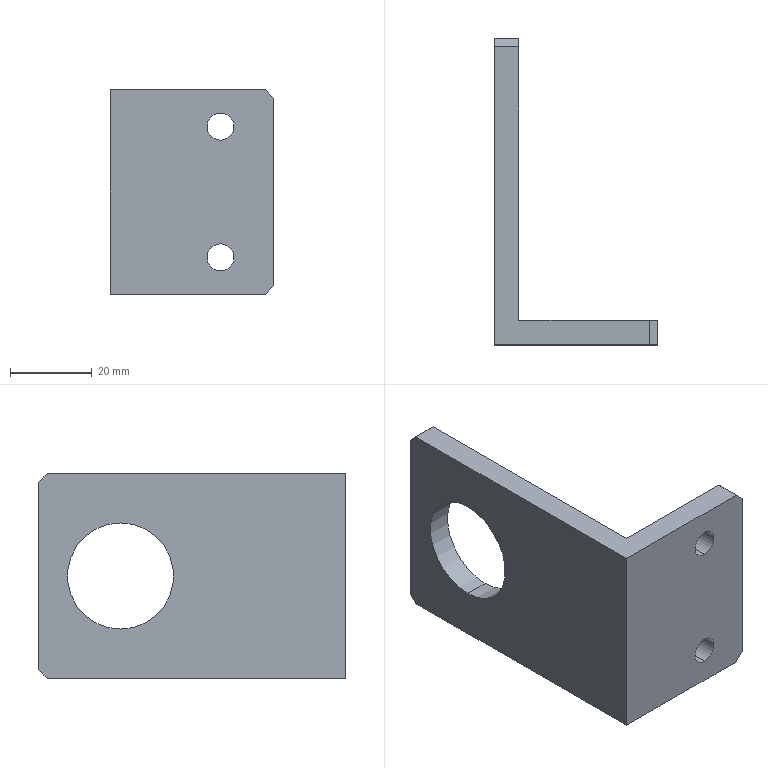Part | SolidWorks | features HoleWzd 2, Chamfer 1, Extrusion 1 | 1 solid | 18 faces | box 40 x 75 x 50 mm | volume 29056 mm3 | plane 12 | cylinder 6 | commonest cylinder face diameters 6.6 x4 26 x2
STEP:
#1=CARTESIAN_POINT('',(-13.82,-27.594,5.7));
#2=VERTEX_POINT('',#1);
#3=CARTESIAN_POINT('',(-13.82,-27.594,12.3));
#4=VERTEX_POINT('',#3);
#5=CARTESIAN_POINT('',(-13.82,-27.594,9.));
#6=DIRECTION('',(0.,1.,0.));
#7=DIRECTION('',(0.,0.,1.));
#8=AXIS2_PLACEMENT_3D('',#5,#6,#7);
#9=CIRCLE('',#8,3.3);
#10=EDGE_CURVE('',#2,#4,#9,.T.);
#11=ORIENTED_EDGE('',*,*,#10,.F.);
#12=CARTESIAN_POINT('',(-13.82,-21.594,5.7));
#13=VERTEX_POINT('',#12);
#14=CARTESIAN_POINT('',(-13.82,-21.594,5.7));
#15=DIRECTION('',(0.,1.,0.));
#16=VECTOR('',#15,1000.);
#17=LINE('',#14,#16);
#18=EDGE_CURVE('',#2,#13,#17,.T.);
#19=ORIENTED_EDGE('',*,*,#18,.T.);
#20=CARTESIAN_POINT('',(-13.82,-21.594,12.3));
#21=VERTEX_POINT('',#20);
#22=CARTESIAN_POINT('',(-13.82,-21.594,9.));
#23=DIRECTION('',(0.,1.,0.));
#24=DIRECTION('',(0.,0.,1.));
#25=AXIS2_PLACEMENT_3D('',#22,#23,#24);
#26=CIRCLE('',#25,3.3);
#27=EDGE_CURVE('',#13,#21,#26,.T.);
#28=ORIENTED_EDGE('',*,*,#27,.T.);
#29=CARTESIAN_POINT('',(-13.82,-21.594,12.3));
#30=DIRECTION('',(0.,1.,0.));
#31=VECTOR('',#30,1000.);
#32=LINE('',#29,#31);
#33=EDGE_CURVE('',#4,#21,#32,.T.);
#34=ORIENTED_EDGE('',*,*,#33,.F.);
#35=EDGE_LOOP('',(#11,#19,#28,#34));
#36=FACE_OUTER_BOUND('',#35,.T.);
#37=CARTESIAN_POINT('',(-13.82,-21.594,9.));
#38=DIRECTION('',(0.,1.,0.));
#39=DIRECTION('',(0.,0.,1.));
#40=AXIS2_PLACEMENT_3D('',#37,#38,#39);
#41=CYLINDRICAL_SURFACE('',#40,3.3);
#42=ADVANCED_FACE('',(#36),#41,.F.);
#43=CARTESIAN_POINT('',(-13.82,-27.594,37.7));
#44=VERTEX_POINT('',#43);
#45=CARTESIAN_POINT('',(-13.82,-27.594,44.3));
#46=VERTEX_POINT('',#45);
#47=CARTESIAN_POINT('',(-13.82,-27.594,41.));
#48=DIRECTION('',(0.,1.,0.));
#49=DIRECTION('',(0.,0.,1.));
#50=AXIS2_PLACEMENT_3D('',#47,#48,#49);
#51=CIRCLE('',#50,3.3);
#52=EDGE_CURVE('',#44,#46,#51,.T.);
#53=ORIENTED_EDGE('',*,*,#52,.F.);
#54=CARTESIAN_POINT('',(-13.82,-21.594,37.7));
#55=VERTEX_POINT('',#54);
#56=CARTESIAN_POINT('',(-13.82,-21.594,37.7));
#57=DIRECTION('',(0.,1.,0.));
#58=VECTOR('',#57,1000.);
#59=LINE('',#56,#58);
#60=EDGE_CURVE('',#44,#55,#59,.T.);
#61=ORIENTED_EDGE('',*,*,#60,.T.);
#62=CARTESIAN_POINT('',(-13.82,-21.594,44.3));
#63=VERTEX_POINT('',#62);
#64=CARTESIAN_POINT('',(-13.82,-21.594,41.));
#65=DIRECTION('',(0.,1.,0.));
#66=DIRECTION('',(0.,0.,1.));
#67=AXIS2_PLACEMENT_3D('',#64,#65,#66);
#68=CIRCLE('',#67,3.3);
#69=EDGE_CURVE('',#55,#63,#68,.T.);
#70=ORIENTED_EDGE('',*,*,#69,.T.);
#71=CARTESIAN_POINT('',(-13.82,-21.594,44.3));
#72=DIRECTION('',(0.,1.,0.));
#73=VECTOR('',#72,1000.);
#74=LINE('',#71,#73);
#75=EDGE_CURVE('',#46,#63,#74,.T.);
#76=ORIENTED_EDGE('',*,*,#75,.F.);
#77=EDGE_LOOP('',(#53,#61,#70,#76));
#78=FACE_OUTER_BOUND('',#77,.T.);
#79=CARTESIAN_POINT('',(-13.82,-21.594,41.));
#80=DIRECTION('',(0.,1.,0.));
#81=DIRECTION('',(0.,0.,1.));
#82=AXIS2_PLACEMENT_3D('',#79,#80,#81);
#83=CYLINDRICAL_SURFACE('',#82,3.3);
#84=ADVANCED_FACE('',(#78),#83,.F.);
#85=CARTESIAN_POINT('',(-40.82,27.406,38.));
#86=VERTEX_POINT('',#85);
#87=CARTESIAN_POINT('',(-40.82,27.406,12.));
#88=VERTEX_POINT('',#87);
#89=CARTESIAN_POINT('',(-40.82,27.406,25.));
#90=DIRECTION('',(1.,0.,0.));
#91=DIRECTION('',(0.,0.,-1.));
#92=AXIS2_PLACEMENT_3D('',#89,#90,#91);
#93=CIRCLE('',#92,13.);
#94=EDGE_CURVE('',#86,#88,#93,.T.);
#95=ORIENTED_EDGE('',*,*,#94,.F.);
#96=CARTESIAN_POINT('',(-34.82,27.406,38.));
#97=VERTEX_POINT('',#96);
#98=CARTESIAN_POINT('',(-34.82,27.406,38.));
#99=DIRECTION('',(1.,0.,0.));
#100=VECTOR('',#99,1000.);
#101=LINE('',#98,#100);
#102=EDGE_CURVE('',#86,#97,#101,.T.);
#103=ORIENTED_EDGE('',*,*,#102,.T.);
#104=CARTESIAN_POINT('',(-34.82,27.406,12.));
#105=VERTEX_POINT('',#104);
#106=CARTESIAN_POINT('',(-34.82,27.406,25.));
#107=DIRECTION('',(1.,0.,0.));
#108=DIRECTION('',(0.,0.,-1.));
#109=AXIS2_PLACEMENT_3D('',#106,#107,#108);
#110=CIRCLE('',#109,13.);
#111=EDGE_CURVE('',#97,#105,#110,.T.);
#112=ORIENTED_EDGE('',*,*,#111,.T.);
#113=CARTESIAN_POINT('',(-34.82,27.406,12.));
#114=DIRECTION('',(1.,0.,0.));
#115=VECTOR('',#114,1000.);
#116=LINE('',#113,#115);
#117=EDGE_CURVE('',#88,#105,#116,.T.);
#118=ORIENTED_EDGE('',*,*,#117,.F.);
#119=EDGE_LOOP('',(#95,#103,#112,#118));
#120=FACE_OUTER_BOUND('',#119,.T.);
#121=CARTESIAN_POINT('',(-34.82,27.406,25.));
#122=DIRECTION('',(1.,0.,0.));
#123=DIRECTION('',(0.,0.,-1.));
#124=AXIS2_PLACEMENT_3D('',#121,#122,#123);
#125=CYLINDRICAL_SURFACE('',#124,13.);
#126=ADVANCED_FACE('',(#120),#125,.F.);
#127=CARTESIAN_POINT('',(-34.82,47.406,48.));
#128=VERTEX_POINT('',#127);
#129=CARTESIAN_POINT('',(-34.82,47.406,2.));
#130=VERTEX_POINT('',#129);
#131=CARTESIAN_POINT('',(-34.82,47.406,50.));
#132=DIRECTION('',(0.,0.,-1.));
#133=VECTOR('',#132,1000.);
#134=LINE('',#131,#133);
#135=EDGE_CURVE('',#128,#130,#134,.T.);
#136=ORIENTED_EDGE('',*,*,#135,.T.);
#137=CARTESIAN_POINT('',(-40.82,47.406,2.));
#138=VERTEX_POINT('',#137);
#139=CARTESIAN_POINT('',(-34.82,47.406,2.));
#140=DIRECTION('',(-1.,0.,0.));
#141=VECTOR('',#140,1000.);
#142=LINE('',#139,#141);
#143=EDGE_CURVE('',#130,#138,#142,.T.);
#144=ORIENTED_EDGE('',*,*,#143,.T.);
#145=CARTESIAN_POINT('',(-40.82,47.406,48.));
#146=VERTEX_POINT('',#145);
#147=CARTESIAN_POINT('',(-40.82,47.406,50.));
#148=DIRECTION('',(0.,0.,-1.));
#149=VECTOR('',#148,1000.);
#150=LINE('',#147,#149);
#151=EDGE_CURVE('',#146,#138,#150,.T.);
#152=ORIENTED_EDGE('',*,*,#151,.F.);
#153=CARTESIAN_POINT('',(-34.82,47.406,48.));
#154=DIRECTION('',(1.,0.,0.));
#155=VECTOR('',#154,1000.);
#156=LINE('',#153,#155);
#157=EDGE_CURVE('',#146,#128,#156,.T.);
#158=ORIENTED_EDGE('',*,*,#157,.T.);
#159=EDGE_LOOP('',(#136,#144,#152,#158));
#160=FACE_OUTER_BOUND('',#159,.T.);
#161=CARTESIAN_POINT('',(-34.82,47.406,50.));
#162=DIRECTION('',(0.,-1.,0.));
#163=DIRECTION('',(0.,0.,-1.));
#164=AXIS2_PLACEMENT_3D('',#161,#162,#163);
#165=PLANE('',#164);
#166=ADVANCED_FACE('',(#160),#165,.F.);
#167=CARTESIAN_POINT('',(-40.82,27.406,25.));
#168=DIRECTION('',(1.,0.,0.));
#169=DIRECTION('',(0.,0.,-1.));
#170=AXIS2_PLACEMENT_3D('',#167,#168,#169);
#171=CIRCLE('',#170,13.);
#172=EDGE_CURVE('',#88,#86,#171,.T.);
#173=ORIENTED_EDGE('',*,*,#172,.T.);
#174=ORIENTED_EDGE('',*,*,#94,.T.);
#175=EDGE_LOOP('',(#173,#174));
#176=FACE_BOUND('',#175,.T.);
#177=ORIENTED_EDGE('',*,*,#151,.T.);
#178=CARTESIAN_POINT('',(-40.82,45.406,0.));
#179=VERTEX_POINT('',#178);
#180=CARTESIAN_POINT('',(-40.82,47.406,2.));
#181=DIRECTION('',(0.,-0.7071,-0.7071));
#182=VECTOR('',#181,1000.);
#183=LINE('',#180,#182);
#184=EDGE_CURVE('',#138,#179,#183,.T.);
#185=ORIENTED_EDGE('',*,*,#184,.T.);
#186=CARTESIAN_POINT('',(-40.82,-27.594,0.));
#187=VERTEX_POINT('',#186);
#188=CARTESIAN_POINT('',(-40.82,47.406,0.));
#189=DIRECTION('',(0.,-1.,0.));
#190=VECTOR('',#189,1000.);
#191=LINE('',#188,#190);
#192=EDGE_CURVE('',#179,#187,#191,.T.);
#193=ORIENTED_EDGE('',*,*,#192,.T.);
#194=CARTESIAN_POINT('',(-40.82,-27.594,50.));
#195=VERTEX_POINT('',#194);
#196=CARTESIAN_POINT('',(-40.82,-27.594,50.));
#197=DIRECTION('',(0.,0.,-1.));
#198=VECTOR('',#197,1000.);
#199=LINE('',#196,#198);
#200=EDGE_CURVE('',#195,#187,#199,.T.);
#201=ORIENTED_EDGE('',*,*,#200,.F.);
#202=CARTESIAN_POINT('',(-40.82,45.406,50.));
#203=VERTEX_POINT('',#202);
#204=CARTESIAN_POINT('',(-40.82,47.406,50.));
#205=DIRECTION('',(0.,-1.,0.));
#206=VECTOR('',#205,1000.);
#207=LINE('',#204,#206);
#208=EDGE_CURVE('',#203,#195,#207,.T.);
#209=ORIENTED_EDGE('',*,*,#208,.F.);
#210=CARTESIAN_POINT('',(-40.82,45.406,50.));
#211=DIRECTION('',(0.,0.7071,-0.7071));
#212=VECTOR('',#211,1000.);
#213=LINE('',#210,#212);
#214=EDGE_CURVE('',#203,#146,#213,.T.);
#215=ORIENTED_EDGE('',*,*,#214,.T.);
#216=EDGE_LOOP('',(#177,#185,#193,#201,#209,#215));
#217=FACE_OUTER_BOUND('',#216,.T.);
#218=CARTESIAN_POINT('',(-40.82,47.406,50.));
#219=DIRECTION('',(1.,0.,0.));
#220=DIRECTION('',(0.,1.,0.));
#221=AXIS2_PLACEMENT_3D('',#218,#219,#220);
#222=PLANE('',#221);
#223=ADVANCED_FACE('',(#176,#217),#222,.F.);
#224=CARTESIAN_POINT('',(-13.82,-27.594,9.));
#225=DIRECTION('',(0.,1.,0.));
#226=DIRECTION('',(0.,0.,1.));
#227=AXIS2_PLACEMENT_3D('',#224,#225,#226);
#228=CIRCLE('',#227,3.3);
#229=EDGE_CURVE('',#4,#2,#228,.T.);
#230=ORIENTED_EDGE('',*,*,#229,.T.);
#231=ORIENTED_EDGE('',*,*,#10,.T.);
#232=EDGE_LOOP('',(#230,#231));
#233=FACE_BOUND('',#232,.T.);
#234=CARTESIAN_POINT('',(-13.82,-27.594,41.));
#235=DIRECTION('',(0.,1.,0.));
#236=DIRECTION('',(0.,0.,1.));
#237=AXIS2_PLACEMENT_3D('',#234,#235,#236);
#238=CIRCLE('',#237,3.3);
#239=EDGE_CURVE('',#46,#44,#238,.T.);
#240=ORIENTED_EDGE('',*,*,#239,.T.);
#241=ORIENTED_EDGE('',*,*,#52,.T.);
#242=EDGE_LOOP('',(#240,#241));
#243=FACE_BOUND('',#242,.T.);
#244=CARTESIAN_POINT('',(-2.82,-27.594,0.));
#245=VERTEX_POINT('',#244);
#246=CARTESIAN_POINT('',(-40.82,-27.594,0.));
#247=DIRECTION('',(1.,0.,0.));
#248=VECTOR('',#247,1000.);
#249=LINE('',#246,#248);
#250=EDGE_CURVE('',#187,#245,#249,.T.);
#251=ORIENTED_EDGE('',*,*,#250,.T.);
#252=CARTESIAN_POINT('',(-0.8198,-27.594,2.));
#253=VERTEX_POINT('',#252);
#254=CARTESIAN_POINT('',(-0.8198,-27.594,2.));
#255=DIRECTION('',(0.7071,0.,0.7071));
#256=VECTOR('',#255,1000.);
#257=LINE('',#254,#256);
#258=EDGE_CURVE('',#245,#253,#257,.T.);
#259=ORIENTED_EDGE('',*,*,#258,.T.);
#260=CARTESIAN_POINT('',(-0.8198,-27.594,48.));
#261=VERTEX_POINT('',#260);
#262=CARTESIAN_POINT('',(-0.8198,-27.594,50.));
#263=DIRECTION('',(0.,0.,-1.));
#264=VECTOR('',#263,1000.);
#265=LINE('',#262,#264);
#266=EDGE_CURVE('',#261,#253,#265,.T.);
#267=ORIENTED_EDGE('',*,*,#266,.F.);
#268=CARTESIAN_POINT('',(-2.82,-27.594,50.));
#269=VERTEX_POINT('',#268);
#270=CARTESIAN_POINT('',(-2.82,-27.594,50.));
#271=DIRECTION('',(-0.7071,0.,0.7071));
#272=VECTOR('',#271,1000.);
#273=LINE('',#270,#272);
#274=EDGE_CURVE('',#261,#269,#273,.T.);
#275=ORIENTED_EDGE('',*,*,#274,.T.);
#276=CARTESIAN_POINT('',(-40.82,-27.594,50.));
#277=DIRECTION('',(1.,0.,0.));
#278=VECTOR('',#277,1000.);
#279=LINE('',#276,#278);
#280=EDGE_CURVE('',#195,#269,#279,.T.);
#281=ORIENTED_EDGE('',*,*,#280,.F.);
#282=ORIENTED_EDGE('',*,*,#200,.T.);
#283=EDGE_LOOP('',(#251,#259,#267,#275,#281,#282));
#284=FACE_OUTER_BOUND('',#283,.T.);
#285=CARTESIAN_POINT('',(-40.82,-27.594,50.));
#286=DIRECTION('',(0.,1.,0.));
#287=DIRECTION('',(0.,0.,1.));
#288=AXIS2_PLACEMENT_3D('',#285,#286,#287);
#289=PLANE('',#288);
#290=ADVANCED_FACE('',(#233,#243,#284),#289,.F.);
#291=ORIENTED_EDGE('',*,*,#266,.T.);
#292=CARTESIAN_POINT('',(-0.8198,-21.594,2.));
#293=VERTEX_POINT('',#292);
#294=CARTESIAN_POINT('',(-0.8198,-27.594,2.));
#295=DIRECTION('',(0.,1.,0.));
#296=VECTOR('',#295,1000.);
#297=LINE('',#294,#296);
#298=EDGE_CURVE('',#253,#293,#297,.T.);
#299=ORIENTED_EDGE('',*,*,#298,.T.);
#300=CARTESIAN_POINT('',(-0.8198,-21.594,48.));
#301=VERTEX_POINT('',#300);
#302=CARTESIAN_POINT('',(-0.8198,-21.594,50.));
#303=DIRECTION('',(0.,0.,-1.));
#304=VECTOR('',#303,1000.);
#305=LINE('',#302,#304);
#306=EDGE_CURVE('',#301,#293,#305,.T.);
#307=ORIENTED_EDGE('',*,*,#306,.F.);
#308=CARTESIAN_POINT('',(-0.8198,-27.594,48.));
#309=DIRECTION('',(0.,-1.,0.));
#310=VECTOR('',#309,1000.);
#311=LINE('',#308,#310);
#312=EDGE_CURVE('',#301,#261,#311,.T.);
#313=ORIENTED_EDGE('',*,*,#312,.T.);
#314=EDGE_LOOP('',(#291,#299,#307,#313));
#315=FACE_OUTER_BOUND('',#314,.T.);
#316=CARTESIAN_POINT('',(-0.8198,-27.594,50.));
#317=DIRECTION('',(-1.,0.,0.));
#318=DIRECTION('',(0.,0.,1.));
#319=AXIS2_PLACEMENT_3D('',#316,#317,#318);
#320=PLANE('',#319);
#321=ADVANCED_FACE('',(#315),#320,.F.);
#322=CARTESIAN_POINT('',(-13.82,-21.594,9.));
#323=DIRECTION('',(0.,1.,0.));
#324=DIRECTION('',(0.,0.,1.));
#325=AXIS2_PLACEMENT_3D('',#322,#323,#324);
#326=CIRCLE('',#325,3.3);
#327=EDGE_CURVE('',#21,#13,#326,.T.);
#328=ORIENTED_EDGE('',*,*,#327,.F.);
#329=ORIENTED_EDGE('',*,*,#27,.F.);
#330=EDGE_LOOP('',(#328,#329));
#331=FACE_BOUND('',#330,.T.);
#332=CARTESIAN_POINT('',(-13.82,-21.594,41.));
#333=DIRECTION('',(0.,1.,0.));
#334=DIRECTION('',(0.,0.,1.));
#335=AXIS2_PLACEMENT_3D('',#332,#333,#334);
#336=CIRCLE('',#335,3.3);
#337=EDGE_CURVE('',#63,#55,#336,.T.);
#338=ORIENTED_EDGE('',*,*,#337,.F.);
#339=ORIENTED_EDGE('',*,*,#69,.F.);
#340=EDGE_LOOP('',(#338,#339));
#341=FACE_BOUND('',#340,.T.);
#342=ORIENTED_EDGE('',*,*,#306,.T.);
#343=CARTESIAN_POINT('',(-2.82,-21.594,0.));
#344=VERTEX_POINT('',#343);
#345=CARTESIAN_POINT('',(-0.8198,-21.594,2.));
#346=DIRECTION('',(-0.7071,0.,-0.7071));
#347=VECTOR('',#346,1000.);
#348=LINE('',#345,#347);
#349=EDGE_CURVE('',#293,#344,#348,.T.);
#350=ORIENTED_EDGE('',*,*,#349,.T.);
#351=CARTESIAN_POINT('',(-34.82,-21.594,0.));
#352=VERTEX_POINT('',#351);
#353=CARTESIAN_POINT('',(-0.8198,-21.594,0.));
#354=DIRECTION('',(-1.,0.,0.));
#355=VECTOR('',#354,1000.);
#356=LINE('',#353,#355);
#357=EDGE_CURVE('',#344,#352,#356,.T.);
#358=ORIENTED_EDGE('',*,*,#357,.T.);
#359=CARTESIAN_POINT('',(-34.82,-21.594,50.));
#360=VERTEX_POINT('',#359);
#361=CARTESIAN_POINT('',(-34.82,-21.594,50.));
#362=DIRECTION('',(0.,0.,-1.));
#363=VECTOR('',#362,1000.);
#364=LINE('',#361,#363);
#365=EDGE_CURVE('',#360,#352,#364,.T.);
#366=ORIENTED_EDGE('',*,*,#365,.F.);
#367=CARTESIAN_POINT('',(-2.82,-21.594,50.));
#368=VERTEX_POINT('',#367);
#369=CARTESIAN_POINT('',(-0.8198,-21.594,50.));
#370=DIRECTION('',(-1.,0.,0.));
#371=VECTOR('',#370,1000.);
#372=LINE('',#369,#371);
#373=EDGE_CURVE('',#368,#360,#372,.T.);
#374=ORIENTED_EDGE('',*,*,#373,.F.);
#375=CARTESIAN_POINT('',(-2.82,-21.594,50.));
#376=DIRECTION('',(0.7071,0.,-0.7071));
#377=VECTOR('',#376,1000.);
#378=LINE('',#375,#377);
#379=EDGE_CURVE('',#368,#301,#378,.T.);
#380=ORIENTED_EDGE('',*,*,#379,.T.);
#381=EDGE_LOOP('',(#342,#350,#358,#366,#374,#380));
#382=FACE_OUTER_BOUND('',#381,.T.);
#383=CARTESIAN_POINT('',(-0.8198,-21.594,50.));
#384=DIRECTION('',(0.,-1.,0.));
#385=DIRECTION('',(1.,0.,0.));
#386=AXIS2_PLACEMENT_3D('',#383,#384,#385);
#387=PLANE('',#386);
#388=ADVANCED_FACE('',(#331,#341,#382),#387,.F.);
#389=CARTESIAN_POINT('',(-34.82,27.406,25.));
#390=DIRECTION('',(1.,0.,0.));
#391=DIRECTION('',(0.,0.,-1.));
#392=AXIS2_PLACEMENT_3D('',#389,#390,#391);
#393=CIRCLE('',#392,13.);
#394=EDGE_CURVE('',#105,#97,#393,.T.);
#395=ORIENTED_EDGE('',*,*,#394,.F.);
#396=ORIENTED_EDGE('',*,*,#111,.F.);
#397=EDGE_LOOP('',(#395,#396));
#398=FACE_BOUND('',#397,.T.);
#399=CARTESIAN_POINT('',(-34.82,45.406,0.));
#400=VERTEX_POINT('',#399);
#401=CARTESIAN_POINT('',(-34.82,-21.594,0.));
#402=DIRECTION('',(0.,1.,0.));
#403=VECTOR('',#402,1000.);
#404=LINE('',#401,#403);
#405=EDGE_CURVE('',#352,#400,#404,.T.);
#406=ORIENTED_EDGE('',*,*,#405,.T.);
#407=CARTESIAN_POINT('',(-34.82,47.406,2.));
#408=DIRECTION('',(0.,0.7071,0.7071));
#409=VECTOR('',#408,1000.);
#410=LINE('',#407,#409);
#411=EDGE_CURVE('',#400,#130,#410,.T.);
#412=ORIENTED_EDGE('',*,*,#411,.T.);
#413=ORIENTED_EDGE('',*,*,#135,.F.);
#414=CARTESIAN_POINT('',(-34.82,45.406,50.));
#415=VERTEX_POINT('',#414);
#416=CARTESIAN_POINT('',(-34.82,45.406,50.));
#417=DIRECTION('',(0.,-0.7071,0.7071));
#418=VECTOR('',#417,1000.);
#419=LINE('',#416,#418);
#420=EDGE_CURVE('',#128,#415,#419,.T.);
#421=ORIENTED_EDGE('',*,*,#420,.T.);
#422=CARTESIAN_POINT('',(-34.82,-21.594,50.));
#423=DIRECTION('',(0.,1.,0.));
#424=VECTOR('',#423,1000.);
#425=LINE('',#422,#424);
#426=EDGE_CURVE('',#360,#415,#425,.T.);
#427=ORIENTED_EDGE('',*,*,#426,.F.);
#428=ORIENTED_EDGE('',*,*,#365,.T.);
#429=EDGE_LOOP('',(#406,#412,#413,#421,#427,#428));
#430=FACE_OUTER_BOUND('',#429,.T.);
#431=CARTESIAN_POINT('',(-34.82,-21.594,50.));
#432=DIRECTION('',(-1.,0.,0.));
#433=DIRECTION('',(0.,0.,1.));
#434=AXIS2_PLACEMENT_3D('',#431,#432,#433);
#435=PLANE('',#434);
#436=ADVANCED_FACE('',(#398,#430),#435,.F.);
#437=ORIENTED_EDGE('',*,*,#280,.T.);
#438=CARTESIAN_POINT('',(-2.82,-21.594,50.));
#439=DIRECTION('',(0.,1.,0.));
#440=VECTOR('',#439,1000.);
#441=LINE('',#438,#440);
#442=EDGE_CURVE('',#269,#368,#441,.T.);
#443=ORIENTED_EDGE('',*,*,#442,.T.);
#444=ORIENTED_EDGE('',*,*,#373,.T.);
#445=ORIENTED_EDGE('',*,*,#426,.T.);
#446=CARTESIAN_POINT('',(-40.82,45.406,50.));
#447=DIRECTION('',(-1.,0.,0.));
#448=VECTOR('',#447,1000.);
#449=LINE('',#446,#448);
#450=EDGE_CURVE('',#415,#203,#449,.T.);
#451=ORIENTED_EDGE('',*,*,#450,.T.);
#452=ORIENTED_EDGE('',*,*,#208,.T.);
#453=EDGE_LOOP('',(#437,#443,#444,#445,#451,#452));
#454=FACE_OUTER_BOUND('',#453,.T.);
#455=CARTESIAN_POINT('',(0.,0.,50.));
#456=DIRECTION('',(0.,0.,1.));
#457=DIRECTION('',(1.,0.,0.));
#458=AXIS2_PLACEMENT_3D('',#455,#456,#457);
#459=PLANE('',#458);
#460=ADVANCED_FACE('',(#454),#459,.T.);
#461=ORIENTED_EDGE('',*,*,#357,.F.);
#462=CARTESIAN_POINT('',(-2.82,0.,0.));
#463=DIRECTION('',(0.,-1.,0.));
#464=VECTOR('',#463,1000.);
#465=LINE('',#462,#464);
#466=EDGE_CURVE('',#344,#245,#465,.T.);
#467=ORIENTED_EDGE('',*,*,#466,.T.);
#468=ORIENTED_EDGE('',*,*,#250,.F.);
#469=ORIENTED_EDGE('',*,*,#192,.F.);
#470=CARTESIAN_POINT('',(0.,45.406,0.));
#471=DIRECTION('',(1.,0.,0.));
#472=VECTOR('',#471,1000.);
#473=LINE('',#470,#472);
#474=EDGE_CURVE('',#179,#400,#473,.T.);
#475=ORIENTED_EDGE('',*,*,#474,.T.);
#476=ORIENTED_EDGE('',*,*,#405,.F.);
#477=EDGE_LOOP('',(#461,#467,#468,#469,#475,#476));
#478=FACE_OUTER_BOUND('',#477,.T.);
#479=CARTESIAN_POINT('',(0.,0.,0.));
#480=DIRECTION('',(0.,0.,1.));
#481=DIRECTION('',(1.,0.,0.));
#482=AXIS2_PLACEMENT_3D('',#479,#480,#481);
#483=PLANE('',#482);
#484=ADVANCED_FACE('',(#478),#483,.F.);
#485=ORIENTED_EDGE('',*,*,#102,.F.);
#486=ORIENTED_EDGE('',*,*,#172,.F.);
#487=ORIENTED_EDGE('',*,*,#117,.T.);
#488=ORIENTED_EDGE('',*,*,#394,.T.);
#489=EDGE_LOOP('',(#485,#486,#487,#488));
#490=FACE_OUTER_BOUND('',#489,.T.);
#491=CARTESIAN_POINT('',(-34.82,27.406,25.));
#492=DIRECTION('',(1.,0.,0.));
#493=DIRECTION('',(0.,0.,-1.));
#494=AXIS2_PLACEMENT_3D('',#491,#492,#493);
#495=CYLINDRICAL_SURFACE('',#494,13.);
#496=ADVANCED_FACE('',(#490),#495,.F.);
#497=ORIENTED_EDGE('',*,*,#258,.F.);
#498=ORIENTED_EDGE('',*,*,#466,.F.);
#499=ORIENTED_EDGE('',*,*,#349,.F.);
#500=ORIENTED_EDGE('',*,*,#298,.F.);
#501=EDGE_LOOP('',(#497,#498,#499,#500));
#502=FACE_OUTER_BOUND('',#501,.T.);
#503=CARTESIAN_POINT('',(-0.8198,-27.594,2.));
#504=DIRECTION('',(-0.7071,0.,0.7071));
#505=DIRECTION('',(0.,1.,0.));
#506=AXIS2_PLACEMENT_3D('',#503,#504,#505);
#507=PLANE('',#506);
#508=ADVANCED_FACE('',(#502),#507,.F.);
#509=ORIENTED_EDGE('',*,*,#274,.F.);
#510=ORIENTED_EDGE('',*,*,#312,.F.);
#511=ORIENTED_EDGE('',*,*,#379,.F.);
#512=ORIENTED_EDGE('',*,*,#442,.F.);
#513=EDGE_LOOP('',(#509,#510,#511,#512));
#514=FACE_OUTER_BOUND('',#513,.T.);
#515=CARTESIAN_POINT('',(-2.82,0.,50.));
#516=DIRECTION('',(0.7071,0.,0.7071));
#517=DIRECTION('',(0.,-1.,0.));
#518=AXIS2_PLACEMENT_3D('',#515,#516,#517);
#519=PLANE('',#518);
#520=ADVANCED_FACE('',(#514),#519,.T.);
#521=ORIENTED_EDGE('',*,*,#411,.F.);
#522=ORIENTED_EDGE('',*,*,#474,.F.);
#523=ORIENTED_EDGE('',*,*,#184,.F.);
#524=ORIENTED_EDGE('',*,*,#143,.F.);
#525=EDGE_LOOP('',(#521,#522,#523,#524));
#526=FACE_OUTER_BOUND('',#525,.T.);
#527=CARTESIAN_POINT('',(-34.82,47.406,2.));
#528=DIRECTION('',(0.,-0.7071,0.7071));
#529=DIRECTION('',(-1.,0.,0.));
#530=AXIS2_PLACEMENT_3D('',#527,#528,#529);
#531=PLANE('',#530);
#532=ADVANCED_FACE('',(#526),#531,.F.);
#533=ORIENTED_EDGE('',*,*,#420,.F.);
#534=ORIENTED_EDGE('',*,*,#157,.F.);
#535=ORIENTED_EDGE('',*,*,#214,.F.);
#536=ORIENTED_EDGE('',*,*,#450,.F.);
#537=EDGE_LOOP('',(#533,#534,#535,#536));
#538=FACE_OUTER_BOUND('',#537,.T.);
#539=CARTESIAN_POINT('',(0.,45.406,50.));
#540=DIRECTION('',(0.,0.7071,0.7071));
#541=DIRECTION('',(1.,0.,0.));
#542=AXIS2_PLACEMENT_3D('',#539,#540,#541);
#543=PLANE('',#542);
#544=ADVANCED_FACE('',(#538),#543,.T.);
#545=ORIENTED_EDGE('',*,*,#60,.F.);
#546=ORIENTED_EDGE('',*,*,#239,.F.);
#547=ORIENTED_EDGE('',*,*,#75,.T.);
#548=ORIENTED_EDGE('',*,*,#337,.T.);
#549=EDGE_LOOP('',(#545,#546,#547,#548));
#550=FACE_OUTER_BOUND('',#549,.T.);
#551=CARTESIAN_POINT('',(-13.82,-21.594,41.));
#552=DIRECTION('',(0.,1.,0.));
#553=DIRECTION('',(0.,0.,1.));
#554=AXIS2_PLACEMENT_3D('',#551,#552,#553);
#555=CYLINDRICAL_SURFACE('',#554,3.3);
#556=ADVANCED_FACE('',(#550),#555,.F.);
#557=ORIENTED_EDGE('',*,*,#18,.F.);
#558=ORIENTED_EDGE('',*,*,#229,.F.);
#559=ORIENTED_EDGE('',*,*,#33,.T.);
#560=ORIENTED_EDGE('',*,*,#327,.T.);
#561=EDGE_LOOP('',(#557,#558,#559,#560));
#562=FACE_OUTER_BOUND('',#561,.T.);
#563=CARTESIAN_POINT('',(-13.82,-21.594,9.));
#564=DIRECTION('',(0.,1.,0.));
#565=DIRECTION('',(0.,0.,1.));
#566=AXIS2_PLACEMENT_3D('',#563,#564,#565);
#567=CYLINDRICAL_SURFACE('',#566,3.3);
#568=ADVANCED_FACE('',(#562),#567,.F.);
#569=CLOSED_SHELL('',(#42,#84,#126,#166,#223,#290,#321,#388,#436,#460,#484,#496,#508,#520,#532,#544,#556,#568));
#570=MANIFOLD_SOLID_BREP('',#569);
#571=CARTESIAN_POINT('',(0.,0.,0.));
#572=DIRECTION('',(0.,0.,1.));
#573=DIRECTION('',(1.,0.,0.));
#574=AXIS2_PLACEMENT_3D('',#571,#572,#573);
#575=(LENGTH_UNIT()NAMED_UNIT(*)SI_UNIT(.MILLI.,.METRE.));
#576=UNCERTAINTY_MEASURE_WITH_UNIT(LENGTH_MEASURE(0.00001),#575,'','');
#577=(NAMED_UNIT(*)PLANE_ANGLE_UNIT()SI_UNIT($,.RADIAN.));
#578=(NAMED_UNIT(*)SI_UNIT($,.STERADIAN.)SOLID_ANGLE_UNIT());
#579=(GEOMETRIC_REPRESENTATION_CONTEXT(3)GLOBAL_UNCERTAINTY_ASSIGNED_CONTEXT((#576))GLOBAL_UNIT_ASSIGNED_CONTEXT((#575,#577,#578))REPRESENTATION_CONTEXT('',''));
#580=ADVANCED_BREP_SHAPE_REPRESENTATION('',(#570,#574),#579);